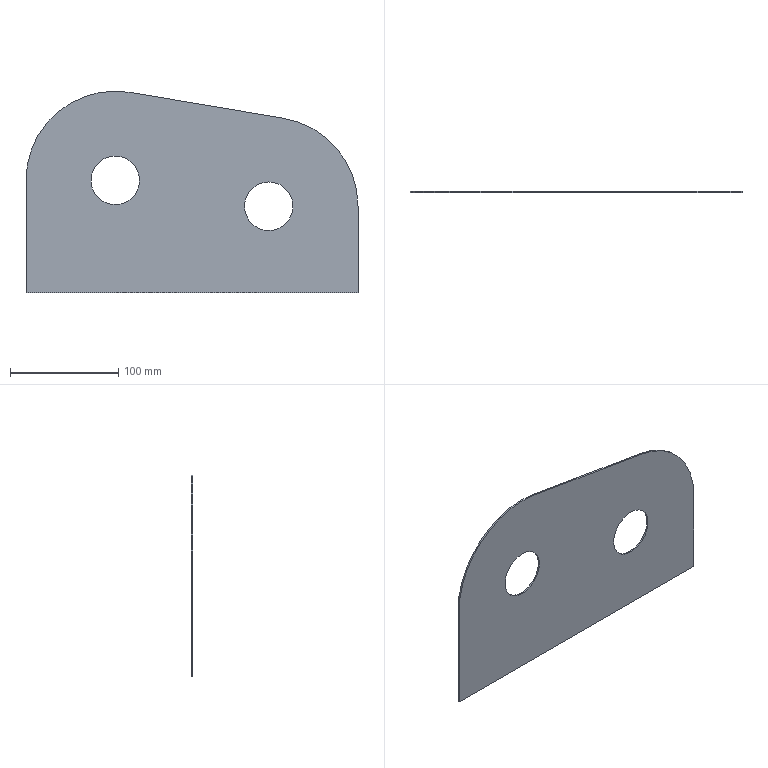Part | STEP file | 冲床-300配套压波_id514_x_t | 1 solid | 10 faces | box 307 x 1.5 x 186.5 mm | volume 71471 mm3 | plane 6 | cylinder 4 | commonest cylinder face diameters 45 x2 165 x2
STEP:
#1=CARTESIAN_POINT('',(1474.5,-135.,0.));
#2=VERTEX_POINT('',#1);
#3=CARTESIAN_POINT('',(1474.5,-133.5,0.));
#4=VERTEX_POINT('',#3);
#5=CARTESIAN_POINT('',(1474.5,-71.5,0.));
#6=DIRECTION('',(0.,1.,0.));
#7=VECTOR('',#6,1.);
#8=LINE('',#5,#7);
#9=EDGE_CURVE('',#2,#4,#8,.T.);
#10=ORIENTED_EDGE('',*,*,#9,.F.);
#11=CARTESIAN_POINT('',(1167.5,-135.,0.));
#12=VERTEX_POINT('',#11);
#13=CARTESIAN_POINT('',(1507.,-135.,0.));
#14=DIRECTION('',(1.,0.,0.));
#15=VECTOR('',#14,1.);
#16=LINE('',#13,#15);
#17=EDGE_CURVE('',#12,#2,#16,.T.);
#18=ORIENTED_EDGE('',*,*,#17,.F.);
#19=CARTESIAN_POINT('',(1167.5,-133.5,0.));
#20=VERTEX_POINT('',#19);
#21=CARTESIAN_POINT('',(1167.5,-71.5,0.));
#22=DIRECTION('',(0.,-1.,0.));
#23=VECTOR('',#22,1.);
#24=LINE('',#21,#23);
#25=EDGE_CURVE('',#20,#12,#24,.T.);
#26=ORIENTED_EDGE('',*,*,#25,.F.);
#27=CARTESIAN_POINT('',(1165.,-133.5,0.));
#28=DIRECTION('',(1.,0.,0.));
#29=VECTOR('',#28,1.);
#30=LINE('',#27,#29);
#31=EDGE_CURVE('',#20,#4,#30,.T.);
#32=ORIENTED_EDGE('',*,*,#31,.T.);
#33=EDGE_LOOP('',(#10,#18,#26,#32));
#34=FACE_OUTER_BOUND('',#33,.T.);
#35=CARTESIAN_POINT('',(1507.,-71.5,0.));
#36=DIRECTION('',(0.,0.,1.));
#37=DIRECTION('',(1.,0.,0.));
#38=AXIS2_PLACEMENT_3D('',#35,#36,#37);
#39=PLANE('',#38);
#40=ADVANCED_FACE('',(#34),#39,.F.);
#41=CARTESIAN_POINT('',(1392.,-133.5,102.583));
#42=VERTEX_POINT('',#41);
#43=CARTESIAN_POINT('',(1392.,-133.5,80.083));
#44=DIRECTION('',(0.,-1.,0.));
#45=DIRECTION('',(0.,0.,1.));
#46=AXIS2_PLACEMENT_3D('',#43,#44,#45);
#47=CIRCLE('',#46,22.5);
#48=EDGE_CURVE('',#42,#42,#47,.T.);
#49=ORIENTED_EDGE('',*,*,#48,.F.);
#50=EDGE_LOOP('',(#49));
#51=FACE_BOUND('',#50,.T.);
#52=CARTESIAN_POINT('',(1392.,-135.,57.583));
#53=VERTEX_POINT('',#52);
#54=CARTESIAN_POINT('',(1392.,-135.,80.083));
#55=DIRECTION('',(0.,-1.,0.));
#56=DIRECTION('',(0.,0.,-1.));
#57=AXIS2_PLACEMENT_3D('',#54,#55,#56);
#58=CIRCLE('',#57,22.5);
#59=EDGE_CURVE('',#53,#53,#58,.T.);
#60=ORIENTED_EDGE('',*,*,#59,.T.);
#61=EDGE_LOOP('',(#60));
#62=FACE_BOUND('',#61,.T.);
#63=CARTESIAN_POINT('',(1392.,-49.5,80.083));
#64=DIRECTION('',(0.,-1.,0.));
#65=DIRECTION('',(0.,0.,1.));
#66=AXIS2_PLACEMENT_3D('',#63,#64,#65);
#67=CYLINDRICAL_SURFACE('',#66,22.5);
#68=ADVANCED_FACE('',(#51,#62),#67,.F.);
#69=CARTESIAN_POINT('',(1250.,-135.,81.5));
#70=VERTEX_POINT('',#69);
#71=CARTESIAN_POINT('',(1250.,-135.,104.));
#72=DIRECTION('',(0.,1.,0.));
#73=DIRECTION('',(0.,0.,-1.));
#74=AXIS2_PLACEMENT_3D('',#71,#72,#73);
#75=CIRCLE('',#74,22.5);
#76=EDGE_CURVE('',#70,#70,#75,.T.);
#77=ORIENTED_EDGE('',*,*,#76,.F.);
#78=EDGE_LOOP('',(#77));
#79=FACE_BOUND('',#78,.T.);
#80=CARTESIAN_POINT('',(1250.,-133.5,126.5));
#81=VERTEX_POINT('',#80);
#82=CARTESIAN_POINT('',(1250.,-133.5,104.));
#83=DIRECTION('',(0.,-1.,0.));
#84=DIRECTION('',(0.,0.,1.));
#85=AXIS2_PLACEMENT_3D('',#82,#83,#84);
#86=CIRCLE('',#85,22.5);
#87=EDGE_CURVE('',#81,#81,#86,.T.);
#88=ORIENTED_EDGE('',*,*,#87,.F.);
#89=EDGE_LOOP('',(#88));
#90=FACE_BOUND('',#89,.T.);
#91=CARTESIAN_POINT('',(1250.,-140.,104.));
#92=DIRECTION('',(0.,1.,0.));
#93=DIRECTION('',(-1.,0.,0.));
#94=AXIS2_PLACEMENT_3D('',#91,#92,#93);
#95=CYLINDRICAL_SURFACE('',#94,22.5);
#96=ADVANCED_FACE('',(#79,#90),#95,.F.);
#97=ORIENTED_EDGE('',*,*,#48,.T.);
#98=EDGE_LOOP('',(#97));
#99=FACE_BOUND('',#98,.T.);
#100=ORIENTED_EDGE('',*,*,#87,.T.);
#101=EDGE_LOOP('',(#100));
#102=FACE_BOUND('',#101,.T.);
#103=ORIENTED_EDGE('',*,*,#31,.F.);
#104=CARTESIAN_POINT('',(1167.5,-133.5,104.));
#105=VERTEX_POINT('',#104);
#106=CARTESIAN_POINT('',(1167.5,-133.5,360.));
#107=DIRECTION('',(0.,0.,1.));
#108=VECTOR('',#107,1.);
#109=LINE('',#106,#108);
#110=EDGE_CURVE('',#20,#105,#109,.T.);
#111=ORIENTED_EDGE('',*,*,#110,.T.);
#112=CARTESIAN_POINT('',(1263.702,-133.5,185.354));
#113=VERTEX_POINT('',#112);
#114=CARTESIAN_POINT('',(1250.,-133.5,104.));
#115=DIRECTION('',(0.,1.,0.));
#116=DIRECTION('',(0.,0.,1.));
#117=AXIS2_PLACEMENT_3D('',#114,#115,#116);
#118=CIRCLE('',#117,82.5);
#119=EDGE_CURVE('',#105,#113,#118,.T.);
#120=ORIENTED_EDGE('',*,*,#119,.T.);
#121=CARTESIAN_POINT('',(1405.702,-133.5,161.438));
#122=VERTEX_POINT('',#121);
#123=CARTESIAN_POINT('',(1139.119,-133.5,206.337));
#124=DIRECTION('',(0.9861,0.,-0.1661));
#125=VECTOR('',#124,1.);
#126=LINE('',#123,#125);
#127=EDGE_CURVE('',#113,#122,#126,.T.);
#128=ORIENTED_EDGE('',*,*,#127,.T.);
#129=CARTESIAN_POINT('',(1474.5,-133.5,80.083));
#130=VERTEX_POINT('',#129);
#131=CARTESIAN_POINT('',(1392.,-133.5,80.083));
#132=DIRECTION('',(0.,-1.,0.));
#133=DIRECTION('',(0.,0.,1.));
#134=AXIS2_PLACEMENT_3D('',#131,#132,#133);
#135=CIRCLE('',#134,82.5);
#136=EDGE_CURVE('',#130,#122,#135,.T.);
#137=ORIENTED_EDGE('',*,*,#136,.F.);
#138=CARTESIAN_POINT('',(1474.5,-133.5,0.));
#139=DIRECTION('',(0.,0.,1.));
#140=VECTOR('',#139,1.);
#141=LINE('',#138,#140);
#142=EDGE_CURVE('',#4,#130,#141,.T.);
#143=ORIENTED_EDGE('',*,*,#142,.F.);
#144=EDGE_LOOP('',(#103,#111,#120,#128,#137,#143));
#145=FACE_BOUND('',#144,.T.);
#146=CARTESIAN_POINT('',(1165.,-133.5,360.));
#147=DIRECTION('',(0.,1.,0.));
#148=DIRECTION('',(0.,0.,1.));
#149=AXIS2_PLACEMENT_3D('',#146,#147,#148);
#150=PLANE('',#149);
#151=ADVANCED_FACE('',(#99,#102,#145),#150,.T.);
#152=ORIENTED_EDGE('',*,*,#76,.T.);
#153=EDGE_LOOP('',(#152));
#154=FACE_BOUND('',#153,.T.);
#155=ORIENTED_EDGE('',*,*,#59,.F.);
#156=EDGE_LOOP('',(#155));
#157=FACE_BOUND('',#156,.T.);
#158=CARTESIAN_POINT('',(1263.702,-135.,185.354));
#159=VERTEX_POINT('',#158);
#160=CARTESIAN_POINT('',(1167.5,-135.,104.));
#161=VERTEX_POINT('',#160);
#162=CARTESIAN_POINT('',(1250.,-135.,104.));
#163=DIRECTION('',(0.,-1.,0.));
#164=DIRECTION('',(0.,0.,-1.));
#165=AXIS2_PLACEMENT_3D('',#162,#163,#164);
#166=CIRCLE('',#165,82.5);
#167=EDGE_CURVE('',#159,#161,#166,.T.);
#168=ORIENTED_EDGE('',*,*,#167,.T.);
#169=CARTESIAN_POINT('',(1167.5,-135.,104.));
#170=DIRECTION('',(0.,0.,-1.));
#171=VECTOR('',#170,1.);
#172=LINE('',#169,#171);
#173=EDGE_CURVE('',#161,#12,#172,.T.);
#174=ORIENTED_EDGE('',*,*,#173,.T.);
#175=ORIENTED_EDGE('',*,*,#17,.T.);
#176=CARTESIAN_POINT('',(1474.5,-135.,80.083));
#177=VERTEX_POINT('',#176);
#178=CARTESIAN_POINT('',(1474.5,-135.,104.));
#179=DIRECTION('',(0.,0.,1.));
#180=VECTOR('',#179,1.);
#181=LINE('',#178,#180);
#182=EDGE_CURVE('',#2,#177,#181,.T.);
#183=ORIENTED_EDGE('',*,*,#182,.T.);
#184=CARTESIAN_POINT('',(1405.702,-135.,161.438));
#185=VERTEX_POINT('',#184);
#186=CARTESIAN_POINT('',(1392.,-135.,80.083));
#187=DIRECTION('',(0.,-1.,0.));
#188=DIRECTION('',(0.,0.,-1.));
#189=AXIS2_PLACEMENT_3D('',#186,#187,#188);
#190=CIRCLE('',#189,82.5);
#191=EDGE_CURVE('',#177,#185,#190,.T.);
#192=ORIENTED_EDGE('',*,*,#191,.T.);
#193=CARTESIAN_POINT('',(1263.702,-135.,185.354));
#194=DIRECTION('',(-0.9861,0.,0.1661));
#195=VECTOR('',#194,1.);
#196=LINE('',#193,#195);
#197=EDGE_CURVE('',#185,#159,#196,.T.);
#198=ORIENTED_EDGE('',*,*,#197,.T.);
#199=EDGE_LOOP('',(#168,#174,#175,#183,#192,#198));
#200=FACE_BOUND('',#199,.T.);
#201=CARTESIAN_POINT('',(1250.,-135.,104.));
#202=DIRECTION('',(0.,-1.,0.));
#203=DIRECTION('',(0.9861,0.,-0.1661));
#204=AXIS2_PLACEMENT_3D('',#201,#202,#203);
#205=PLANE('',#204);
#206=ADVANCED_FACE('',(#154,#157,#200),#205,.T.);
#207=ORIENTED_EDGE('',*,*,#173,.F.);
#208=CARTESIAN_POINT('',(1167.5,-400.5,104.));
#209=DIRECTION('',(0.,1.,0.));
#210=VECTOR('',#209,1.);
#211=LINE('',#208,#210);
#212=EDGE_CURVE('',#161,#105,#211,.T.);
#213=ORIENTED_EDGE('',*,*,#212,.T.);
#214=ORIENTED_EDGE('',*,*,#110,.F.);
#215=ORIENTED_EDGE('',*,*,#25,.T.);
#216=EDGE_LOOP('',(#207,#213,#214,#215));
#217=FACE_OUTER_BOUND('',#216,.T.);
#218=CARTESIAN_POINT('',(1167.5,133.,104.));
#219=DIRECTION('',(-1.,0.,0.));
#220=DIRECTION('',(0.,0.,1.));
#221=AXIS2_PLACEMENT_3D('',#218,#219,#220);
#222=PLANE('',#221);
#223=ADVANCED_FACE('',(#217),#222,.T.);
#224=ORIENTED_EDGE('',*,*,#142,.T.);
#225=CARTESIAN_POINT('',(1474.5,-400.5,80.083));
#226=DIRECTION('',(0.,1.,0.));
#227=VECTOR('',#226,1.);
#228=LINE('',#225,#227);
#229=EDGE_CURVE('',#177,#130,#228,.T.);
#230=ORIENTED_EDGE('',*,*,#229,.F.);
#231=ORIENTED_EDGE('',*,*,#182,.F.);
#232=ORIENTED_EDGE('',*,*,#9,.T.);
#233=EDGE_LOOP('',(#224,#230,#231,#232));
#234=FACE_OUTER_BOUND('',#233,.T.);
#235=CARTESIAN_POINT('',(1474.5,133.,0.));
#236=DIRECTION('',(1.,0.,0.));
#237=DIRECTION('',(0.,0.,-1.));
#238=AXIS2_PLACEMENT_3D('',#235,#236,#237);
#239=PLANE('',#238);
#240=ADVANCED_FACE('',(#234),#239,.T.);
#241=ORIENTED_EDGE('',*,*,#127,.F.);
#242=CARTESIAN_POINT('',(1263.702,-400.5,185.354));
#243=DIRECTION('',(0.,1.,0.));
#244=VECTOR('',#243,1.);
#245=LINE('',#242,#244);
#246=EDGE_CURVE('',#159,#113,#245,.T.);
#247=ORIENTED_EDGE('',*,*,#246,.F.);
#248=ORIENTED_EDGE('',*,*,#197,.F.);
#249=CARTESIAN_POINT('',(1405.702,-400.5,161.438));
#250=DIRECTION('',(0.,1.,0.));
#251=VECTOR('',#250,1.);
#252=LINE('',#249,#251);
#253=EDGE_CURVE('',#185,#122,#252,.T.);
#254=ORIENTED_EDGE('',*,*,#253,.T.);
#255=EDGE_LOOP('',(#241,#247,#248,#254));
#256=FACE_OUTER_BOUND('',#255,.T.);
#257=CARTESIAN_POINT('',(1263.702,-400.5,185.354));
#258=DIRECTION('',(0.1661,0.,0.9861));
#259=DIRECTION('',(0.9861,0.,-0.1661));
#260=AXIS2_PLACEMENT_3D('',#257,#258,#259);
#261=PLANE('',#260);
#262=ADVANCED_FACE('',(#256),#261,.T.);
#263=ORIENTED_EDGE('',*,*,#119,.F.);
#264=ORIENTED_EDGE('',*,*,#212,.F.);
#265=ORIENTED_EDGE('',*,*,#167,.F.);
#266=ORIENTED_EDGE('',*,*,#246,.T.);
#267=EDGE_LOOP('',(#263,#264,#265,#266));
#268=FACE_OUTER_BOUND('',#267,.T.);
#269=CARTESIAN_POINT('',(1250.,-400.5,104.));
#270=DIRECTION('',(0.,1.,0.));
#271=DIRECTION('',(0.,0.,1.));
#272=AXIS2_PLACEMENT_3D('',#269,#270,#271);
#273=CYLINDRICAL_SURFACE('',#272,82.5);
#274=ADVANCED_FACE('',(#268),#273,.T.);
#275=ORIENTED_EDGE('',*,*,#229,.T.);
#276=ORIENTED_EDGE('',*,*,#136,.T.);
#277=ORIENTED_EDGE('',*,*,#253,.F.);
#278=ORIENTED_EDGE('',*,*,#191,.F.);
#279=EDGE_LOOP('',(#275,#276,#277,#278));
#280=FACE_OUTER_BOUND('',#279,.T.);
#281=CARTESIAN_POINT('',(1392.,-400.5,80.083));
#282=DIRECTION('',(0.,1.,0.));
#283=DIRECTION('',(0.,0.,1.));
#284=AXIS2_PLACEMENT_3D('',#281,#282,#283);
#285=CYLINDRICAL_SURFACE('',#284,82.5);
#286=ADVANCED_FACE('',(#280),#285,.T.);
#287=CLOSED_SHELL('',(#40,#68,#96,#151,#206,#223,#240,#262,#274,#286));
#288=MANIFOLD_SOLID_BREP('',#287);
#289=(LENGTH_UNIT()NAMED_UNIT(*)SI_UNIT(.MILLI.,.METRE.));
#290=UNCERTAINTY_MEASURE_WITH_UNIT(LENGTH_MEASURE(0.00002),#289,'','');
#291=(NAMED_UNIT(*)PLANE_ANGLE_UNIT()SI_UNIT($,.RADIAN.));
#292=PLANE_ANGLE_MEASURE_WITH_UNIT(PLANE_ANGLE_MEASURE(0.01745),#291);
#293=DIMENSIONAL_EXPONENTS(0.,0.,0.,0.,0.,0.,0.);
#294=(CONVERSION_BASED_UNIT('DEGREE',#292)NAMED_UNIT(#293)PLANE_ANGLE_UNIT());
#295=(NAMED_UNIT(*)SI_UNIT($,.STERADIAN.)SOLID_ANGLE_UNIT());
#296=(GEOMETRIC_REPRESENTATION_CONTEXT(3)GLOBAL_UNCERTAINTY_ASSIGNED_CONTEXT((#290))GLOBAL_UNIT_ASSIGNED_CONTEXT((#289,#294,#295))REPRESENTATION_CONTEXT('',''));
#297=ADVANCED_BREP_SHAPE_REPRESENTATION('',(#288),#296);